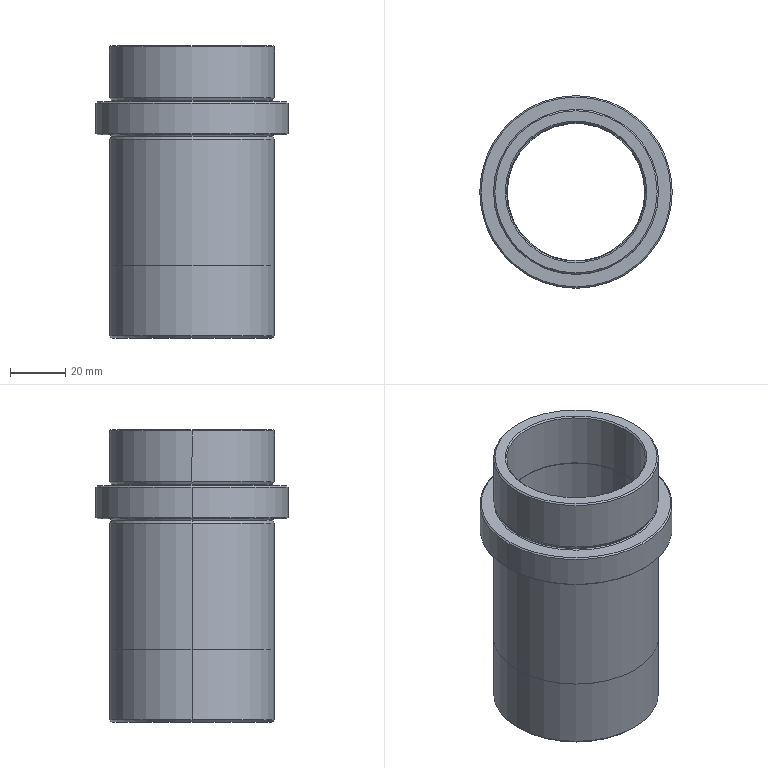Part | STEP file | Bushing BG - PN_0002 - cut | 1 solid | 41 faces | box 70 x 70 x 106.5 mm | volume 102431 mm3 | cone 14 | cylinder 12 | torus 10 | plane 5 | commonest cylinder face diameters 60 x4 50 x2 50.5 x2 59.98 x2 70 x2